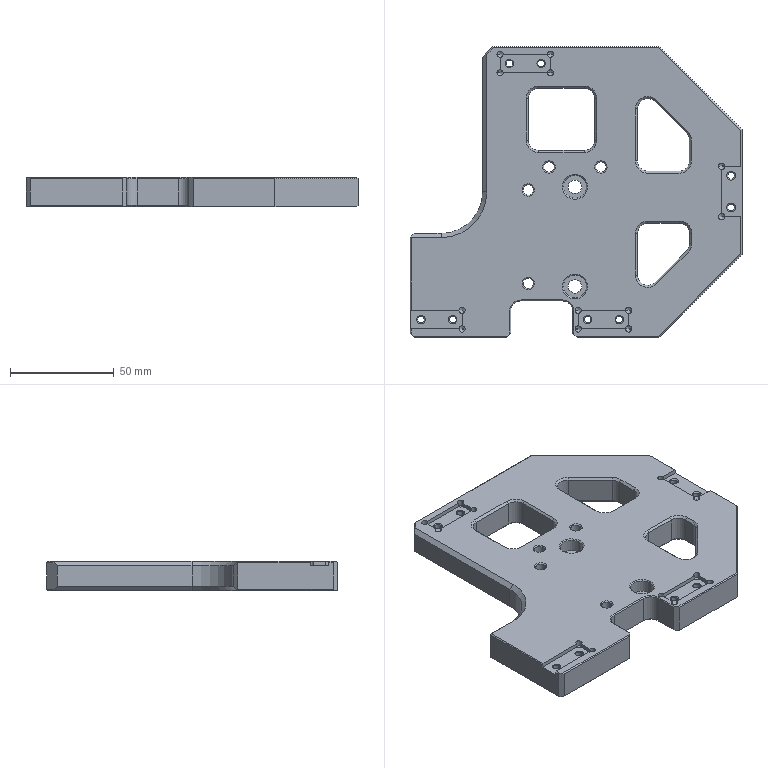Part | SolidWorks | features Chamfer 3, Cut 2, HoleWzd 2, BaseBody 1, DelFace 1, LibraryFeature 1 | 1 solid | 262 faces | box 160 x 140 x 14 mm | volume 203256 mm3 | plane 101 | cone 90 | cylinder 71 | commonest cylinder face diameters 3 x24 3.3 x16 10 x14 5 x8 6.5 x4 11 x4